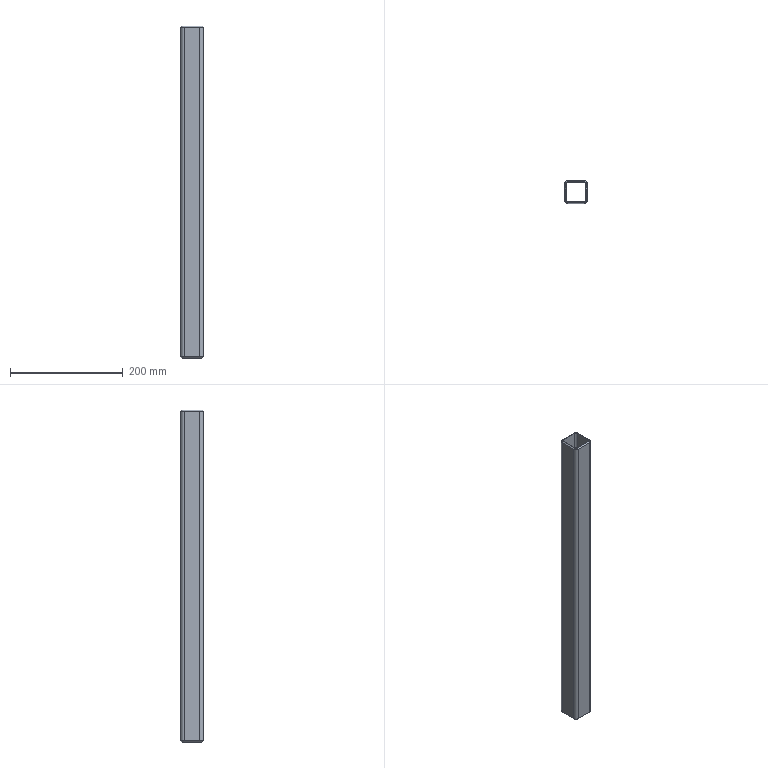Part | STEP file | IN-01-01-01-06 | 1 solid | 36 faces | box 40 x 40 x 590 mm | volume 240323 mm3 | plane 18 | cylinder 10 | cone 8 | commonest cylinder face diameters 5.8 x4 11.6 x4 10 x2